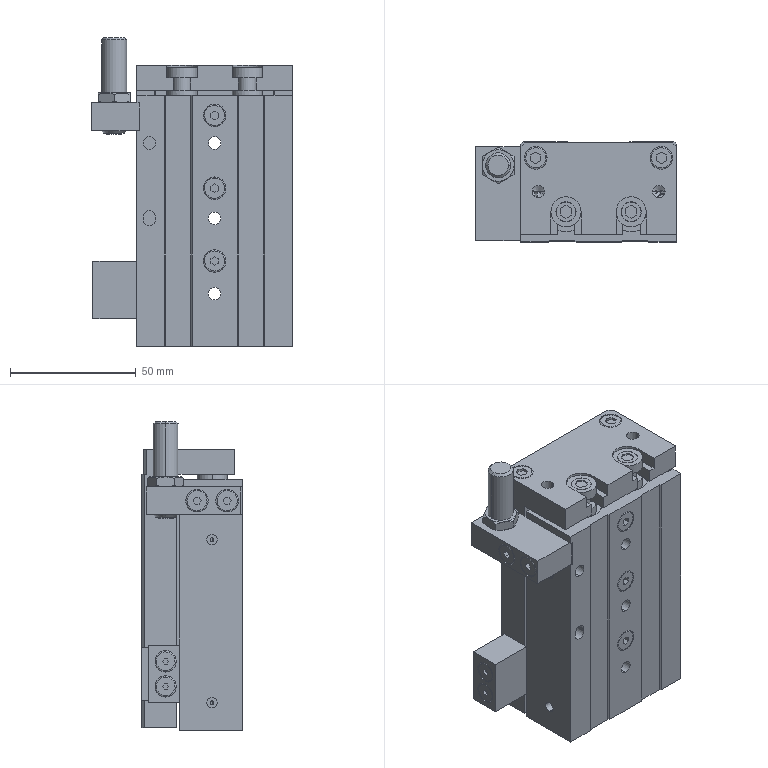Part | SolidWorks | features BaseBody 6, HoleWzd 2, LibraryFeature 2, MoveFace 1 | 6 solids | 516 faces | box 80 x 40 x 123 mm | volume 242427 mm3 | plane 302 | cylinder 167 | spline 24 | cone 23 | commonest cylinder face diameters 5 x35 4.134 x32 16 x16 9 x14 7 x10 12 x8